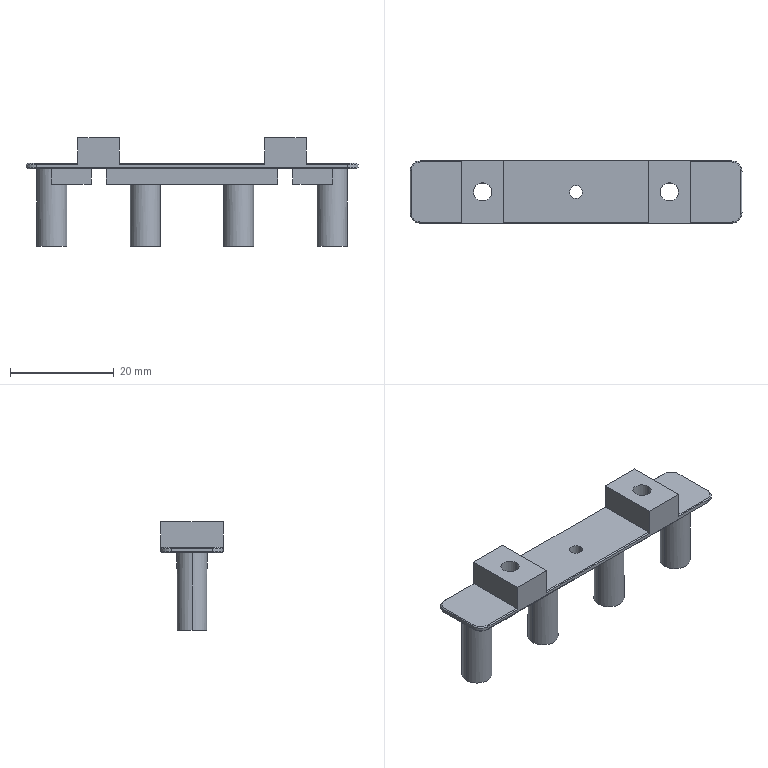NC program | NX | posted with a generic post | part box 64 x 12 x 21 mm
Lines 1897 to 2110 of 2110:
(ZLEVEL_PROFILE_1 , TOOL : D10JING)
N3762 T14 M6
N3764 G54
N3766 G17 G0 G90 X-31.679 Y12.942 S9500 M3
N3768 G43 Z30. H14
N3770 Z-9.
N3772 G94 G1 Z-10.5 F1000.
N3774 G41 X-31.645 Y12.848 D14
N3776 X-30.866 Y11.5
N3778 G3 X-30. Y11. R1.
N3780 G1 X30. F1500.
N3782 G2 X37. Y4. R7.
N3784 G1 Y-4.
N3786 G2 X30. Y-11. R7.
N3788 G1 X-30.
N3790 G2 X-37. Y-4. R7.
N3792 G1 Y4.
N3794 G2 X-30. Y11. R7.
N3796 G1 X30. Z-14.001
N3798 X30.366 Y10.99 Z-14.022
N3800 X30.732 Y10.962 Z-14.043
N3802 X31.095 Y10.914 Z-14.065
N3804 X31.455 Y10.847 Z-14.086
N3806 X31.812 Y10.761 Z-14.108
N3808 X32.163 Y10.657 Z-14.129
N3810 X32.509 Y10.535 Z-14.15
N3812 X32.847 Y10.395 Z-14.172
N3814 X33.178 Y10.237 Z-14.193
N3816 X33.5 Y10.062 Z-14.214
N3818 X33.812 Y9.871 Z-14.236
N3820 X34.114 Y9.663 Z-14.257
N3822 X34.405 Y9.44 Z-14.279
N3824 X34.684 Y9.202 Z-14.3
N3826 X34.95 Y8.95 Z-14.321
N3828 X35.202 Y8.684 Z-14.343
N3830 X35.44 Y8.405 Z-14.364
N3832 X35.663 Y8.114 Z-14.385
N3834 X35.871 Y7.812 Z-14.407
N3836 X36.062 Y7.5 Z-14.428
N3838 X36.237 Y7.178 Z-14.45
N3840 X36.395 Y6.847 Z-14.471
N3842 X36.535 Y6.509 Z-14.492
N3844 X36.657 Y6.163 Z-14.514
N3846 X36.761 Y5.812 Z-14.535
N3848 X36.847 Y5.455 Z-14.556
N3850 X36.914 Y5.095 Z-14.578
N3852 X36.962 Y4.732 Z-14.599
N3854 X36.99 Y4.366 Z-14.621
N3856 X37. Y4. Z-14.642
N3858 Y-4. Z-15.109
N3860 X36.99 Y-4.366 Z-15.13
N3862 X36.962 Y-4.732 Z-15.152
N3864 X36.914 Y-5.095 Z-15.173
N3866 X36.847 Y-5.455 Z-15.194
N3868 X36.761 Y-5.812 Z-15.216
N3870 X36.657 Y-6.163 Z-15.237
N3872 X36.535 Y-6.509 Z-15.258
N3874 X36.395 Y-6.847 Z-15.28
N3876 X36.237 Y-7.178 Z-15.301
N3878 X36.062 Y-7.5 Z-15.323
N3880 X35.871 Y-7.812 Z-15.344
N3882 X35.663 Y-8.114 Z-15.365
N3884 X35.44 Y-8.405 Z-15.387
N3886 X35.202 Y-8.684 Z-15.408
N3888 X34.95 Y-8.95 Z-15.429
N3890 X34.684 Y-9.202 Z-15.451
N3892 X34.405 Y-9.44 Z-15.472
N3894 X34.114 Y-9.663 Z-15.494
N3896 X33.812 Y-9.871 Z-15.515
N3898 X33.5 Y-10.062 Z-15.536
N3900 X33.178 Y-10.237 Z-15.558
N3902 X32.847 Y-10.395 Z-15.579
N3904 X32.509 Y-10.535 Z-15.6
N3906 X32.163 Y-10.657 Z-15.622
N3908 X31.812 Y-10.761 Z-15.643
N3910 X31.455 Y-10.847 Z-15.665
N3912 X31.095 Y-10.914 Z-15.686
N3914 X30.732 Y-10.962 Z-15.707
N3916 X30.366 Y-10.99 Z-15.729
N3918 X30. Y-11. Z-15.75
N3920 X-30. Z-19.251
N3922 X-30.366 Y-10.99 Z-19.272
N3924 X-30.732 Y-10.962 Z-19.293
N3926 X-31.095 Y-10.914 Z-19.315
N3928 X-31.455 Y-10.847 Z-19.336
N3930 X-31.812 Y-10.761 Z-19.358
N3932 X-32.163 Y-10.657 Z-19.379
N3934 X-32.509 Y-10.535 Z-19.4
N3936 X-32.847 Y-10.395 Z-19.422
N3938 X-33.178 Y-10.237 Z-19.443
N3940 X-33.5 Y-10.062 Z-19.464
N3942 X-33.812 Y-9.871 Z-19.486
N3944 X-34.114 Y-9.663 Z-19.507
N3946 X-34.405 Y-9.44 Z-19.529
N3948 X-34.684 Y-9.202 Z-19.55
N3950 X-34.95 Y-8.95 Z-19.571
N3952 X-35.202 Y-8.684 Z-19.593
N3954 X-35.44 Y-8.405 Z-19.614
N3956 X-35.663 Y-8.114 Z-19.635
N3958 X-35.871 Y-7.812 Z-19.657
N3960 X-36.062 Y-7.5 Z-19.678
N3962 X-36.237 Y-7.178 Z-19.7
N3964 X-36.395 Y-6.847 Z-19.721
N3966 X-36.535 Y-6.509 Z-19.742
N3968 X-36.657 Y-6.163 Z-19.764
N3970 X-36.761 Y-5.812 Z-19.785
N3972 X-36.847 Y-5.455 Z-19.806
N3974 X-36.914 Y-5.095 Z-19.828
N3976 X-36.962 Y-4.732 Z-19.849
N3978 X-36.99 Y-4.366 Z-19.871
N3980 X-37. Y-4. Z-19.892
N3982 Y4. Z-20.359
N3984 X-36.99 Y4.366 Z-20.38
N3986 X-36.962 Y4.732 Z-20.402
N3988 X-36.914 Y5.095 Z-20.423
N3990 X-36.847 Y5.455 Z-20.444
N3992 X-36.761 Y5.812 Z-20.466
N3994 X-36.657 Y6.163 Z-20.487
N3996 X-36.535 Y6.509 Z-20.508
N3998 X-36.395 Y6.847 Z-20.53
N4000 X-36.237 Y7.178 Z-20.551
N4002 X-36.062 Y7.5 Z-20.573
N4004 X-35.871 Y7.812 Z-20.594
N4006 X-35.663 Y8.114 Z-20.615
N4008 X-35.44 Y8.405 Z-20.637
N4010 X-35.202 Y8.684 Z-20.658
N4012 X-34.95 Y8.95 Z-20.679
N4014 X-34.684 Y9.202 Z-20.701
N4016 X-34.405 Y9.44 Z-20.722
N4018 X-34.114 Y9.663 Z-20.744
N4020 X-33.812 Y9.871 Z-20.765
N4022 X-33.5 Y10.062 Z-20.786
N4024 X-33.178 Y10.237 Z-20.808
N4026 X-32.847 Y10.395 Z-20.829
N4028 X-32.509 Y10.535 Z-20.85
N4030 X-32.163 Y10.657 Z-20.872
N4032 X-31.812 Y10.761 Z-20.893
N4034 X-31.455 Y10.847 Z-20.915
N4036 X-31.095 Y10.914 Z-20.936
N4038 X-30.732 Y10.962 Z-20.957
N4040 X-30.366 Y10.99 Z-20.979
N4042 X-30. Y11. Z-21.
N4044 X30.
N4046 G2 X37. Y4. R7.
N4048 G1 Y-4.
N4050 G2 X30. Y-11. R7.
N4052 G1 X-30.
N4054 G2 X-37. Y-4. R7.
N4056 G1 Y4.
N4058 G2 X-30. Y11. R7.
N4060 G3 X-29.134 Y11.5 R1.
N4062 G1 X-28.268 Y13.
N4064 G40
N4066 X-28.234 Y13.094
N4068 Z-19.5
N4070 G0 Z30.
(PLANAR_MILL_COPY_COPY_COPY , TOOL : D6A45)
N4072 T01 M6
N4074 G17 G43 G0 G90 X23.4 Y0.866 Z30. S9500 H1 M3
N4076 Z0.5
N4078 G94 G1 Z-1. F1250.
N4080 G3 X22.9 Y0. R1.
N4082 G1 Y-6.
N4084 G2 X22. Y-6.9 R0.9
N4086 G1 X14.
N4088 G2 X13.1 Y-6. R0.9
N4090 G1 Y6.
N4092 G2 X14. Y6.9 R0.9
N4094 G1 X22.
N4096 G2 X22.9 Y6. R0.9
N4098 G1 Y0.
N4100 G3 X23.4 Y-0.866 R1.
N4102 G1 Z0.5
N4104 G0 Z30.
N4106 X18.6 Y-0.433
N4108 Z0.5
N4110 G1 Z-1.
N4112 G3 X18.85 Y0. R0.5
N4114 X18. Y0.85 R0.85
N4116 X18.85 Y0. R-0.85
N4118 X18.6 Y0.433 R0.5
N4120 G1 Z0.5
N4122 G0 Z30.
N4124 X-23.4 Y-0.866
N4126 Z0.5
N4128 G1 Z-1.
N4130 G3 X-22.9 Y0. R1.
N4132 G1 Y6.
N4134 G2 X-22. Y6.9 R0.9
N4136 G1 X-14.
N4138 G2 X-13.1 Y6. R0.9
N4140 G1 Y-6.
N4142 G2 X-14. Y-6.9 R0.9
N4144 G1 X-22.
N4146 G2 X-22.9 Y-6. R0.9
N4148 G1 Y0.
N4150 G3 X-23.4 Y0.866 R1.
N4152 G1 Z0.5
N4154 G0 Z30.
N4156 X-18.6 Y0.433
N4158 Z0.5
N4160 G1 Z-1.
N4162 G3 X-18.85 Y0. R0.5
N4164 X-18. Y-0.85 R0.85
N4166 X-18.85 Y0. R-0.85
N4168 X-18.6 Y-0.433 R0.5
N4170 G1 Z0.5
N4172 G0 Z30.
N4174 M5
N4176 M2